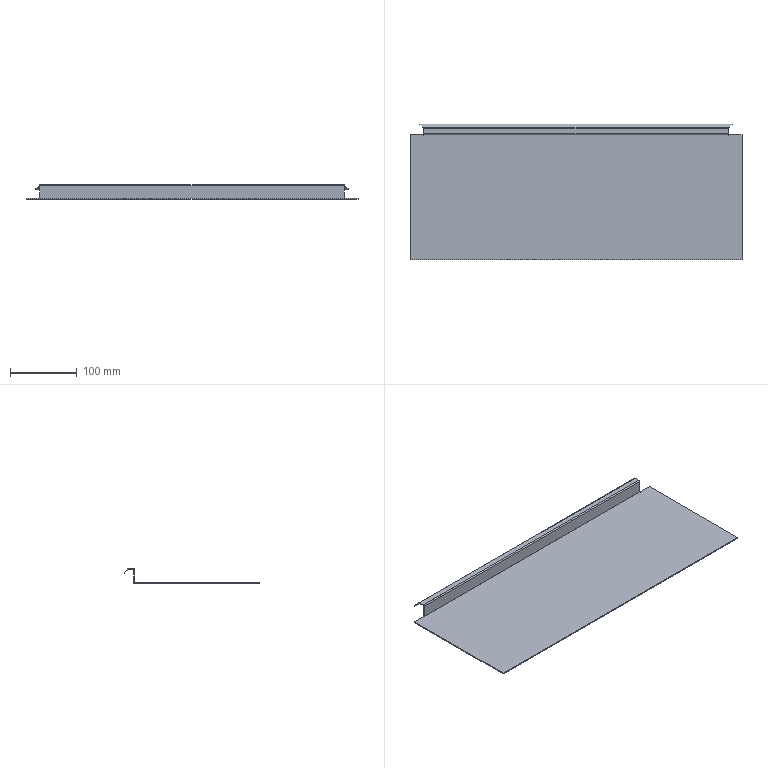Part | SolidWorks | features EdgeFlange 3, SMBaseFlange 2, FlatPattern 1, SheetMetal 1 | 1 solid | 40 faces | box 496.5 x 203.157 x 22 mm | volume 165083 mm3 | plane 34 | cylinder 6 | commonest cylinder face diameters 0.2 x3 3.2 x3
STEP:
#1=CARTESIAN_POINT('',(227.95,103.087,19.));
#2=VERTEX_POINT('',#1);
#3=CARTESIAN_POINT('',(227.95,103.087,20.5));
#4=VERTEX_POINT('',#3);
#5=CARTESIAN_POINT('',(227.95,103.087,19.));
#6=DIRECTION('',(0.,0.,1.));
#7=VECTOR('',#6,1000.);
#8=LINE('',#5,#7);
#9=EDGE_CURVE('',#2,#4,#8,.T.);
#10=ORIENTED_EDGE('',*,*,#9,.T.);
#11=CARTESIAN_POINT('',(227.95,95.35,20.5));
#12=VERTEX_POINT('',#11);
#13=CARTESIAN_POINT('',(227.95,95.25,20.5));
#14=DIRECTION('',(0.,1.,0.));
#15=VECTOR('',#14,1000.);
#16=LINE('',#13,#15);
#17=EDGE_CURVE('',#12,#4,#16,.T.);
#18=ORIENTED_EDGE('',*,*,#17,.F.);
#19=CARTESIAN_POINT('',(227.95,95.35,19.));
#20=VERTEX_POINT('',#19);
#21=CARTESIAN_POINT('',(227.95,95.35,19.));
#22=DIRECTION('',(0.,0.,1.));
#23=VECTOR('',#22,1000.);
#24=LINE('',#21,#23);
#25=EDGE_CURVE('',#20,#12,#24,.T.);
#26=ORIENTED_EDGE('',*,*,#25,.F.);
#27=CARTESIAN_POINT('',(227.95,103.75,19.));
#28=DIRECTION('',(0.,1.,0.));
#29=VECTOR('',#28,1000.);
#30=LINE('',#27,#29);
#31=EDGE_CURVE('',#20,#2,#30,.T.);
#32=ORIENTED_EDGE('',*,*,#31,.T.);
#33=EDGE_LOOP('',(#10,#18,#26,#32));
#34=FACE_OUTER_BOUND('',#33,.T.);
#35=CARTESIAN_POINT('',(227.95,103.75,20.5));
#36=DIRECTION('',(-1.,0.,0.));
#37=DIRECTION('',(0.,0.,1.));
#38=AXIS2_PLACEMENT_3D('',#35,#36,#37);
#39=PLANE('',#38);
#40=ADVANCED_FACE('',(#34),#39,.F.);
#41=CARTESIAN_POINT('',(-227.95,103.087,19.));
#42=VERTEX_POINT('',#41);
#43=CARTESIAN_POINT('',(-227.95,103.087,20.5));
#44=VERTEX_POINT('',#43);
#45=CARTESIAN_POINT('',(-227.95,103.087,19.));
#46=DIRECTION('',(0.,0.,1.));
#47=VECTOR('',#46,1000.);
#48=LINE('',#45,#47);
#49=EDGE_CURVE('',#42,#44,#48,.T.);
#50=ORIENTED_EDGE('',*,*,#49,.F.);
#51=CARTESIAN_POINT('',(-227.95,95.35,19.));
#52=VERTEX_POINT('',#51);
#53=CARTESIAN_POINT('',(-227.95,95.25,19.));
#54=DIRECTION('',(0.,-1.,0.));
#55=VECTOR('',#54,1000.);
#56=LINE('',#53,#55);
#57=EDGE_CURVE('',#42,#52,#56,.T.);
#58=ORIENTED_EDGE('',*,*,#57,.T.);
#59=CARTESIAN_POINT('',(-227.95,95.35,20.5));
#60=VERTEX_POINT('',#59);
#61=CARTESIAN_POINT('',(-227.95,95.35,20.5));
#62=DIRECTION('',(0.,0.,1.));
#63=VECTOR('',#62,1000.);
#64=LINE('',#61,#63);
#65=EDGE_CURVE('',#52,#60,#64,.T.);
#66=ORIENTED_EDGE('',*,*,#65,.T.);
#67=CARTESIAN_POINT('',(-227.95,95.25,20.5));
#68=DIRECTION('',(0.,-1.,0.));
#69=VECTOR('',#68,1000.);
#70=LINE('',#67,#69);
#71=EDGE_CURVE('',#44,#60,#70,.T.);
#72=ORIENTED_EDGE('',*,*,#71,.F.);
#73=EDGE_LOOP('',(#50,#58,#66,#72));
#74=FACE_OUTER_BOUND('',#73,.T.);
#75=CARTESIAN_POINT('',(-227.95,95.25,20.5));
#76=DIRECTION('',(1.,0.,0.));
#77=DIRECTION('',(0.,0.,-1.));
#78=AXIS2_PLACEMENT_3D('',#75,#76,#77);
#79=PLANE('',#78);
#80=ADVANCED_FACE('',(#74),#79,.F.);
#81=CARTESIAN_POINT('',(227.95,103.087,20.5));
#82=DIRECTION('',(-1.,0.,0.));
#83=VECTOR('',#82,1000.);
#84=LINE('',#81,#83);
#85=EDGE_CURVE('',#4,#44,#84,.T.);
#86=ORIENTED_EDGE('',*,*,#85,.T.);
#87=ORIENTED_EDGE('',*,*,#71,.T.);
#88=CARTESIAN_POINT('',(-227.95,95.35,20.5));
#89=DIRECTION('',(-1.,0.,0.));
#90=VECTOR('',#89,1000.);
#91=LINE('',#88,#90);
#92=EDGE_CURVE('',#12,#60,#91,.T.);
#93=ORIENTED_EDGE('',*,*,#92,.F.);
#94=ORIENTED_EDGE('',*,*,#17,.T.);
#95=EDGE_LOOP('',(#86,#87,#93,#94));
#96=FACE_OUTER_BOUND('',#95,.T.);
#97=CARTESIAN_POINT('',(-227.95,95.25,20.5));
#98=DIRECTION('',(0.,0.,-1.));
#99=DIRECTION('',(-1.,0.,0.));
#100=AXIS2_PLACEMENT_3D('',#97,#98,#99);
#101=PLANE('',#100);
#102=ADVANCED_FACE('',(#96),#101,.F.);
#103=ORIENTED_EDGE('',*,*,#57,.F.);
#104=CARTESIAN_POINT('',(227.95,103.087,19.));
#105=DIRECTION('',(-1.,0.,0.));
#106=VECTOR('',#105,1000.);
#107=LINE('',#104,#106);
#108=EDGE_CURVE('',#2,#42,#107,.T.);
#109=ORIENTED_EDGE('',*,*,#108,.F.);
#110=ORIENTED_EDGE('',*,*,#31,.F.);
#111=CARTESIAN_POINT('',(-227.95,95.35,19.));
#112=DIRECTION('',(1.,0.,0.));
#113=VECTOR('',#112,1000.);
#114=LINE('',#111,#113);
#115=EDGE_CURVE('',#52,#20,#114,.T.);
#116=ORIENTED_EDGE('',*,*,#115,.F.);
#117=EDGE_LOOP('',(#103,#109,#110,#116));
#118=FACE_OUTER_BOUND('',#117,.T.);
#119=CARTESIAN_POINT('',(-227.95,95.25,19.));
#120=DIRECTION('',(0.,0.,-1.));
#121=DIRECTION('',(-1.,0.,0.));
#122=AXIS2_PLACEMENT_3D('',#119,#120,#121);
#123=PLANE('',#122);
#124=ADVANCED_FACE('',(#118),#123,.T.);
#125=CARTESIAN_POINT('',(227.95,95.25,0.1));
#126=VERTEX_POINT('',#125);
#127=CARTESIAN_POINT('',(227.95,95.25,18.9));
#128=VERTEX_POINT('',#127);
#129=CARTESIAN_POINT('',(227.95,95.25,20.5));
#130=DIRECTION('',(0.,0.,1.));
#131=VECTOR('',#130,1000.);
#132=LINE('',#129,#131);
#133=EDGE_CURVE('',#126,#128,#132,.T.);
#134=ORIENTED_EDGE('',*,*,#133,.T.);
#135=CARTESIAN_POINT('',(227.95,93.75,18.9));
#136=VERTEX_POINT('',#135);
#137=CARTESIAN_POINT('',(227.95,95.25,18.9));
#138=DIRECTION('',(0.,-1.,0.));
#139=VECTOR('',#138,1000.);
#140=LINE('',#137,#139);
#141=EDGE_CURVE('',#128,#136,#140,.T.);
#142=ORIENTED_EDGE('',*,*,#141,.T.);
#143=CARTESIAN_POINT('',(227.95,93.75,0.1));
#144=VERTEX_POINT('',#143);
#145=CARTESIAN_POINT('',(227.95,93.75,20.5));
#146=DIRECTION('',(0.,0.,1.));
#147=VECTOR('',#146,1000.);
#148=LINE('',#145,#147);
#149=EDGE_CURVE('',#144,#136,#148,.T.);
#150=ORIENTED_EDGE('',*,*,#149,.F.);
#151=CARTESIAN_POINT('',(227.95,93.75,0.1));
#152=DIRECTION('',(0.,1.,0.));
#153=VECTOR('',#152,1000.);
#154=LINE('',#151,#153);
#155=EDGE_CURVE('',#144,#126,#154,.T.);
#156=ORIENTED_EDGE('',*,*,#155,.T.);
#157=EDGE_LOOP('',(#134,#142,#150,#156));
#158=FACE_OUTER_BOUND('',#157,.T.);
#159=CARTESIAN_POINT('',(227.95,95.25,20.5));
#160=DIRECTION('',(1.,0.,0.));
#161=DIRECTION('',(0.,0.,-1.));
#162=AXIS2_PLACEMENT_3D('',#159,#160,#161);
#163=PLANE('',#162);
#164=ADVANCED_FACE('',(#158),#163,.T.);
#165=CARTESIAN_POINT('',(-227.95,95.25,18.9));
#166=VERTEX_POINT('',#165);
#167=CARTESIAN_POINT('',(-227.95,95.25,0.1));
#168=VERTEX_POINT('',#167);
#169=CARTESIAN_POINT('',(-227.95,95.25,0.));
#170=DIRECTION('',(0.,0.,-1.));
#171=VECTOR('',#170,1000.);
#172=LINE('',#169,#171);
#173=EDGE_CURVE('',#166,#168,#172,.T.);
#174=ORIENTED_EDGE('',*,*,#173,.F.);
#175=CARTESIAN_POINT('',(227.95,95.25,18.9));
#176=DIRECTION('',(-1.,0.,0.));
#177=VECTOR('',#176,1000.);
#178=LINE('',#175,#177);
#179=EDGE_CURVE('',#128,#166,#178,.T.);
#180=ORIENTED_EDGE('',*,*,#179,.F.);
#181=ORIENTED_EDGE('',*,*,#133,.F.);
#182=CARTESIAN_POINT('',(-227.95,95.25,0.1));
#183=DIRECTION('',(-1.,0.,0.));
#184=VECTOR('',#183,1000.);
#185=LINE('',#182,#184);
#186=EDGE_CURVE('',#126,#168,#185,.T.);
#187=ORIENTED_EDGE('',*,*,#186,.T.);
#188=EDGE_LOOP('',(#174,#180,#181,#187));
#189=FACE_OUTER_BOUND('',#188,.T.);
#190=CARTESIAN_POINT('',(-227.95,95.25,0.));
#191=DIRECTION('',(0.,1.,0.));
#192=DIRECTION('',(0.,0.,1.));
#193=AXIS2_PLACEMENT_3D('',#190,#191,#192);
#194=PLANE('',#193);
#195=ADVANCED_FACE('',(#189),#194,.T.);
#196=CARTESIAN_POINT('',(-227.95,93.75,18.9));
#197=VERTEX_POINT('',#196);
#198=CARTESIAN_POINT('',(227.95,93.75,18.9));
#199=DIRECTION('',(-1.,0.,0.));
#200=VECTOR('',#199,1000.);
#201=LINE('',#198,#200);
#202=EDGE_CURVE('',#136,#197,#201,.T.);
#203=ORIENTED_EDGE('',*,*,#202,.T.);
#204=CARTESIAN_POINT('',(-227.95,93.75,0.1));
#205=VERTEX_POINT('',#204);
#206=CARTESIAN_POINT('',(-227.95,93.75,0.));
#207=DIRECTION('',(0.,0.,-1.));
#208=VECTOR('',#207,1000.);
#209=LINE('',#206,#208);
#210=EDGE_CURVE('',#197,#205,#209,.T.);
#211=ORIENTED_EDGE('',*,*,#210,.T.);
#212=CARTESIAN_POINT('',(227.95,93.75,0.1));
#213=DIRECTION('',(-1.,0.,0.));
#214=VECTOR('',#213,1000.);
#215=LINE('',#212,#214);
#216=EDGE_CURVE('',#144,#205,#215,.T.);
#217=ORIENTED_EDGE('',*,*,#216,.F.);
#218=ORIENTED_EDGE('',*,*,#149,.T.);
#219=EDGE_LOOP('',(#203,#211,#217,#218));
#220=FACE_OUTER_BOUND('',#219,.T.);
#221=CARTESIAN_POINT('',(-227.95,93.75,0.));
#222=DIRECTION('',(0.,1.,0.));
#223=DIRECTION('',(0.,0.,1.));
#224=AXIS2_PLACEMENT_3D('',#221,#222,#223);
#225=PLANE('',#224);
#226=ADVANCED_FACE('',(#220),#225,.F.);
#227=CARTESIAN_POINT('',(-228.7,93.75,0.));
#228=VERTEX_POINT('',#227);
#229=CARTESIAN_POINT('',(-248.25,93.75,0.));
#230=VERTEX_POINT('',#229);
#231=CARTESIAN_POINT('',(-248.25,93.75,0.));
#232=DIRECTION('',(-1.,0.,0.));
#233=VECTOR('',#232,1000.);
#234=LINE('',#231,#233);
#235=EDGE_CURVE('',#228,#230,#234,.T.);
#236=ORIENTED_EDGE('',*,*,#235,.F.);
#237=CARTESIAN_POINT('',(-228.7,93.75,-1.5));
#238=VERTEX_POINT('',#237);
#239=CARTESIAN_POINT('',(-228.7,93.75,0.));
#240=DIRECTION('',(0.,0.,-1.));
#241=VECTOR('',#240,1000.);
#242=LINE('',#239,#241);
#243=EDGE_CURVE('',#228,#238,#242,.T.);
#244=ORIENTED_EDGE('',*,*,#243,.T.);
#245=CARTESIAN_POINT('',(-248.25,93.75,-1.5));
#246=VERTEX_POINT('',#245);
#247=CARTESIAN_POINT('',(-248.25,93.75,-1.5));
#248=DIRECTION('',(-1.,0.,0.));
#249=VECTOR('',#248,1000.);
#250=LINE('',#247,#249);
#251=EDGE_CURVE('',#238,#246,#250,.T.);
#252=ORIENTED_EDGE('',*,*,#251,.T.);
#253=CARTESIAN_POINT('',(-248.25,93.75,-1.5));
#254=DIRECTION('',(0.,0.,1.));
#255=VECTOR('',#254,1000.);
#256=LINE('',#253,#255);
#257=EDGE_CURVE('',#246,#230,#256,.T.);
#258=ORIENTED_EDGE('',*,*,#257,.T.);
#259=EDGE_LOOP('',(#236,#244,#252,#258));
#260=FACE_OUTER_BOUND('',#259,.T.);
#261=CARTESIAN_POINT('',(-248.25,93.75,-1.5));
#262=DIRECTION('',(0.,1.,0.));
#263=DIRECTION('',(0.,0.,1.));
#264=AXIS2_PLACEMENT_3D('',#261,#262,#263);
#265=PLANE('',#264);
#266=ADVANCED_FACE('',(#260),#265,.T.);
#267=CARTESIAN_POINT('',(248.25,93.75,-1.5));
#268=VERTEX_POINT('',#267);
#269=CARTESIAN_POINT('',(228.7,93.75,-1.5));
#270=VERTEX_POINT('',#269);
#271=CARTESIAN_POINT('',(-248.25,93.75,-1.5));
#272=DIRECTION('',(-1.,0.,0.));
#273=VECTOR('',#272,1000.);
#274=LINE('',#271,#273);
#275=EDGE_CURVE('',#268,#270,#274,.T.);
#276=ORIENTED_EDGE('',*,*,#275,.T.);
#277=CARTESIAN_POINT('',(228.7,93.75,0.));
#278=VERTEX_POINT('',#277);
#279=CARTESIAN_POINT('',(228.7,93.75,0.));
#280=DIRECTION('',(0.,0.,-1.));
#281=VECTOR('',#280,1000.);
#282=LINE('',#279,#281);
#283=EDGE_CURVE('',#278,#270,#282,.T.);
#284=ORIENTED_EDGE('',*,*,#283,.F.);
#285=CARTESIAN_POINT('',(248.25,93.75,0.));
#286=VERTEX_POINT('',#285);
#287=CARTESIAN_POINT('',(-248.25,93.75,0.));
#288=DIRECTION('',(-1.,0.,0.));
#289=VECTOR('',#288,1000.);
#290=LINE('',#287,#289);
#291=EDGE_CURVE('',#286,#278,#290,.T.);
#292=ORIENTED_EDGE('',*,*,#291,.F.);
#293=CARTESIAN_POINT('',(248.25,93.75,-1.5));
#294=DIRECTION('',(0.,0.,1.));
#295=VECTOR('',#294,1000.);
#296=LINE('',#293,#295);
#297=EDGE_CURVE('',#268,#286,#296,.T.);
#298=ORIENTED_EDGE('',*,*,#297,.F.);
#299=EDGE_LOOP('',(#276,#284,#292,#298));
#300=FACE_OUTER_BOUND('',#299,.T.);
#301=CARTESIAN_POINT('',(-248.25,93.75,-1.5));
#302=DIRECTION('',(0.,1.,0.));
#303=DIRECTION('',(0.,0.,1.));
#304=AXIS2_PLACEMENT_3D('',#301,#302,#303);
#305=PLANE('',#304);
#306=ADVANCED_FACE('',(#300),#305,.T.);
#307=CARTESIAN_POINT('',(-228.7,92.9,-1.5));
#308=VERTEX_POINT('',#307);
#309=CARTESIAN_POINT('',(-228.7,-93.75,-1.5));
#310=DIRECTION('',(0.,1.,0.));
#311=VECTOR('',#310,1000.);
#312=LINE('',#309,#311);
#313=EDGE_CURVE('',#308,#238,#312,.T.);
#314=ORIENTED_EDGE('',*,*,#313,.F.);
#315=CARTESIAN_POINT('',(-227.95,92.9,-1.5));
#316=VERTEX_POINT('',#315);
#317=CARTESIAN_POINT('',(248.25,92.9,-1.5));
#318=DIRECTION('',(-1.,0.,0.));
#319=VECTOR('',#318,1000.);
#320=LINE('',#317,#319);
#321=EDGE_CURVE('',#316,#308,#320,.T.);
#322=ORIENTED_EDGE('',*,*,#321,.F.);
#323=CARTESIAN_POINT('',(-227.95,93.65,-1.5));
#324=VERTEX_POINT('',#323);
#325=CARTESIAN_POINT('',(-227.95,-93.75,-1.5));
#326=DIRECTION('',(0.,-1.,0.));
#327=VECTOR('',#326,1000.);
#328=LINE('',#325,#327);
#329=EDGE_CURVE('',#324,#316,#328,.T.);
#330=ORIENTED_EDGE('',*,*,#329,.F.);
#331=CARTESIAN_POINT('',(227.95,93.65,-1.5));
#332=VERTEX_POINT('',#331);
#333=CARTESIAN_POINT('',(-227.95,93.65,-1.5));
#334=DIRECTION('',(1.,0.,0.));
#335=VECTOR('',#334,1000.);
#336=LINE('',#333,#335);
#337=EDGE_CURVE('',#324,#332,#336,.T.);
#338=ORIENTED_EDGE('',*,*,#337,.T.);
#339=CARTESIAN_POINT('',(227.95,92.9,-1.5));
#340=VERTEX_POINT('',#339);
#341=CARTESIAN_POINT('',(227.95,-93.75,-1.5));
#342=DIRECTION('',(0.,1.,0.));
#343=VECTOR('',#342,1000.);
#344=LINE('',#341,#343);
#345=EDGE_CURVE('',#340,#332,#344,.T.);
#346=ORIENTED_EDGE('',*,*,#345,.F.);
#347=CARTESIAN_POINT('',(228.7,92.9,-1.5));
#348=VERTEX_POINT('',#347);
#349=CARTESIAN_POINT('',(248.25,92.9,-1.5));
#350=DIRECTION('',(-1.,0.,0.));
#351=VECTOR('',#350,1000.);
#352=LINE('',#349,#351);
#353=EDGE_CURVE('',#348,#340,#352,.T.);
#354=ORIENTED_EDGE('',*,*,#353,.F.);
#355=CARTESIAN_POINT('',(228.7,-93.75,-1.5));
#356=DIRECTION('',(0.,-1.,0.));
#357=VECTOR('',#356,1000.);
#358=LINE('',#355,#357);
#359=EDGE_CURVE('',#270,#348,#358,.T.);
#360=ORIENTED_EDGE('',*,*,#359,.F.);
#361=ORIENTED_EDGE('',*,*,#275,.F.);
#362=CARTESIAN_POINT('',(248.25,-93.75,-1.5));
#363=VERTEX_POINT('',#362);
#364=CARTESIAN_POINT('',(248.25,93.75,-1.5));
#365=DIRECTION('',(0.,1.,0.));
#366=VECTOR('',#365,1000.);
#367=LINE('',#364,#366);
#368=EDGE_CURVE('',#363,#268,#367,.T.);
#369=ORIENTED_EDGE('',*,*,#368,.F.);
#370=CARTESIAN_POINT('',(-248.25,-93.75,-1.5));
#371=VERTEX_POINT('',#370);
#372=CARTESIAN_POINT('',(-248.25,-93.75,-1.5));
#373=DIRECTION('',(1.,0.,0.));
#374=VECTOR('',#373,1000.);
#375=LINE('',#372,#374);
#376=EDGE_CURVE('',#371,#363,#375,.T.);
#377=ORIENTED_EDGE('',*,*,#376,.F.);
#378=CARTESIAN_POINT('',(-248.25,93.75,-1.5));
#379=DIRECTION('',(0.,-1.,0.));
#380=VECTOR('',#379,1000.);
#381=LINE('',#378,#380);
#382=EDGE_CURVE('',#246,#371,#381,.T.);
#383=ORIENTED_EDGE('',*,*,#382,.F.);
#384=ORIENTED_EDGE('',*,*,#251,.F.);
#385=EDGE_LOOP('',(#314,#322,#330,#338,#346,#354,#360,#361,#369,#377,#383,#384));
#386=FACE_OUTER_BOUND('',#385,.T.);
#387=CARTESIAN_POINT('',(248.25,-93.75,-1.5));
#388=DIRECTION('',(0.,0.,1.));
#389=DIRECTION('',(1.,0.,0.));
#390=AXIS2_PLACEMENT_3D('',#387,#388,#389);
#391=PLANE('',#390);
#392=ADVANCED_FACE('',(#386),#391,.F.);
#393=CARTESIAN_POINT('',(-228.7,92.9,0.));
#394=VERTEX_POINT('',#393);
#395=CARTESIAN_POINT('',(-227.95,92.9,0.));
#396=VERTEX_POINT('',#395);
#397=CARTESIAN_POINT('',(-228.7,92.9,0.));
#398=DIRECTION('',(1.,0.,0.));
#399=VECTOR('',#398,1000.);
#400=LINE('',#397,#399);
#401=EDGE_CURVE('',#394,#396,#400,.T.);
#402=ORIENTED_EDGE('',*,*,#401,.F.);
#403=CARTESIAN_POINT('',(-228.7,93.75,0.));
#404=DIRECTION('',(0.,-1.,0.));
#405=VECTOR('',#404,1000.);
#406=LINE('',#403,#405);
#407=EDGE_CURVE('',#228,#394,#406,.T.);
#408=ORIENTED_EDGE('',*,*,#407,.F.);
#409=ORIENTED_EDGE('',*,*,#235,.T.);
#410=CARTESIAN_POINT('',(-248.25,-93.75,0.));
#411=VERTEX_POINT('',#410);
#412=CARTESIAN_POINT('',(-248.25,93.75,0.));
#413=DIRECTION('',(0.,-1.,0.));
#414=VECTOR('',#413,1000.);
#415=LINE('',#412,#414);
#416=EDGE_CURVE('',#230,#411,#415,.T.);
#417=ORIENTED_EDGE('',*,*,#416,.T.);
#418=CARTESIAN_POINT('',(248.25,-93.75,0.));
#419=VERTEX_POINT('',#418);
#420=CARTESIAN_POINT('',(-248.25,-93.75,0.));
#421=DIRECTION('',(1.,0.,0.));
#422=VECTOR('',#421,1000.);
#423=LINE('',#420,#422);
#424=EDGE_CURVE('',#411,#419,#423,.T.);
#425=ORIENTED_EDGE('',*,*,#424,.T.);
#426=CARTESIAN_POINT('',(248.25,93.75,0.));
#427=DIRECTION('',(0.,1.,0.));
#428=VECTOR('',#427,1000.);
#429=LINE('',#426,#428);
#430=EDGE_CURVE('',#419,#286,#429,.T.);
#431=ORIENTED_EDGE('',*,*,#430,.T.);
#432=ORIENTED_EDGE('',*,*,#291,.T.);
#433=CARTESIAN_POINT('',(228.7,92.9,0.));
#434=VERTEX_POINT('',#433);
#435=CARTESIAN_POINT('',(228.7,92.9,0.));
#436=DIRECTION('',(0.,1.,0.));
#437=VECTOR('',#436,1000.);
#438=LINE('',#435,#437);
#439=EDGE_CURVE('',#434,#278,#438,.T.);
#440=ORIENTED_EDGE('',*,*,#439,.F.);
#441=CARTESIAN_POINT('',(227.95,92.9,0.));
#442=VERTEX_POINT('',#441);
#443=CARTESIAN_POINT('',(227.95,92.9,0.));
#444=DIRECTION('',(1.,0.,0.));
#445=VECTOR('',#444,1000.);
#446=LINE('',#443,#445);
#447=EDGE_CURVE('',#442,#434,#446,.T.);
#448=ORIENTED_EDGE('',*,*,#447,.F.);
#449=CARTESIAN_POINT('',(227.95,93.65,0.));
#450=VERTEX_POINT('',#449);
#451=CARTESIAN_POINT('',(227.95,93.65,0.));
#452=DIRECTION('',(0.,-1.,0.));
#453=VECTOR('',#452,1000.);
#454=LINE('',#451,#453);
#455=EDGE_CURVE('',#450,#442,#454,.T.);
#456=ORIENTED_EDGE('',*,*,#455,.F.);
#457=CARTESIAN_POINT('',(-227.95,93.65,0.));
#458=VERTEX_POINT('',#457);
#459=CARTESIAN_POINT('',(-227.95,93.65,0.));
#460=DIRECTION('',(1.,0.,0.));
#461=VECTOR('',#460,1000.);
#462=LINE('',#459,#461);
#463=EDGE_CURVE('',#458,#450,#462,.T.);
#464=ORIENTED_EDGE('',*,*,#463,.F.);
#465=CARTESIAN_POINT('',(-227.95,92.9,0.));
#466=DIRECTION('',(0.,1.,0.));
#467=VECTOR('',#466,1000.);
#468=LINE('',#465,#467);
#469=EDGE_CURVE('',#396,#458,#468,.T.);
#470=ORIENTED_EDGE('',*,*,#469,.F.);
#471=EDGE_LOOP('',(#402,#408,#409,#417,#425,#431,#432,#440,#448,#456,#464,#470));
#472=FACE_OUTER_BOUND('',#471,.T.);
#473=CARTESIAN_POINT('',(248.25,-93.75,0.));
#474=DIRECTION('',(0.,0.,1.));
#475=DIRECTION('',(1.,0.,0.));
#476=AXIS2_PLACEMENT_3D('',#473,#474,#475);
#477=PLANE('',#476);
#478=ADVANCED_FACE('',(#472),#477,.T.);
#479=ORIENTED_EDGE('',*,*,#430,.F.);
#480=CARTESIAN_POINT('',(248.25,-93.75,-1.5));
#481=DIRECTION('',(0.,0.,1.));
#482=VECTOR('',#481,1000.);
#483=LINE('',#480,#482);
#484=EDGE_CURVE('',#363,#419,#483,.T.);
#485=ORIENTED_EDGE('',*,*,#484,.F.);
#486=ORIENTED_EDGE('',*,*,#368,.T.);
#487=ORIENTED_EDGE('',*,*,#297,.T.);
#488=EDGE_LOOP('',(#479,#485,#486,#487));
#489=FACE_OUTER_BOUND('',#488,.T.);
#490=CARTESIAN_POINT('',(248.25,93.75,-1.5));
#491=DIRECTION('',(1.,0.,0.));
#492=DIRECTION('',(0.,0.,-1.));
#493=AXIS2_PLACEMENT_3D('',#490,#491,#492);
#494=PLANE('',#493);
#495=ADVANCED_FACE('',(#489),#494,.T.);
#496=ORIENTED_EDGE('',*,*,#424,.F.);
#497=CARTESIAN_POINT('',(-248.25,-93.75,-1.5));
#498=DIRECTION('',(0.,0.,1.));
#499=VECTOR('',#498,1000.);
#500=LINE('',#497,#499);
#501=EDGE_CURVE('',#371,#411,#500,.T.);
#502=ORIENTED_EDGE('',*,*,#501,.F.);
#503=ORIENTED_EDGE('',*,*,#376,.T.);
#504=ORIENTED_EDGE('',*,*,#484,.T.);
#505=EDGE_LOOP('',(#496,#502,#503,#504));
#506=FACE_OUTER_BOUND('',#505,.T.);
#507=CARTESIAN_POINT('',(-248.25,-93.75,-1.5));
#508=DIRECTION('',(0.,-1.,0.));
#509=DIRECTION('',(0.,0.,-1.));
#510=AXIS2_PLACEMENT_3D('',#507,#508,#509);
#511=PLANE('',#510);
#512=ADVANCED_FACE('',(#506),#511,.T.);
#513=ORIENTED_EDGE('',*,*,#416,.F.);
#514=ORIENTED_EDGE('',*,*,#257,.F.);
#515=ORIENTED_EDGE('',*,*,#382,.T.);
#516=ORIENTED_EDGE('',*,*,#501,.T.);
#517=EDGE_LOOP('',(#513,#514,#515,#516));
#518=FACE_OUTER_BOUND('',#517,.T.);
#519=CARTESIAN_POINT('',(-248.25,93.75,-1.5));
#520=DIRECTION('',(-1.,0.,0.));
#521=DIRECTION('',(0.,-1.,0.));
#522=AXIS2_PLACEMENT_3D('',#519,#520,#521);
#523=PLANE('',#522);
#524=ADVANCED_FACE('',(#518),#523,.T.);
#525=CARTESIAN_POINT('',(-228.7,92.9,0.));
#526=DIRECTION('',(0.,0.,-1.));
#527=VECTOR('',#526,1000.);
#528=LINE('',#525,#527);
#529=EDGE_CURVE('',#394,#308,#528,.T.);
#530=ORIENTED_EDGE('',*,*,#529,.T.);
#531=ORIENTED_EDGE('',*,*,#313,.T.);
#532=ORIENTED_EDGE('',*,*,#243,.F.);
#533=ORIENTED_EDGE('',*,*,#407,.T.);
#534=EDGE_LOOP('',(#530,#531,#532,#533));
#535=FACE_OUTER_BOUND('',#534,.T.);
#536=CARTESIAN_POINT('',(-228.7,93.75,0.));
#537=DIRECTION('',(1.,0.,0.));
#538=DIRECTION('',(0.,0.,-1.));
#539=AXIS2_PLACEMENT_3D('',#536,#537,#538);
#540=PLANE('',#539);
#541=ADVANCED_FACE('',(#535),#540,.T.);
#542=CARTESIAN_POINT('',(-227.95,92.9,0.));
#543=DIRECTION('',(0.,0.,-1.));
#544=VECTOR('',#543,1000.);
#545=LINE('',#542,#544);
#546=EDGE_CURVE('',#396,#316,#545,.T.);
#547=ORIENTED_EDGE('',*,*,#546,.T.);
#548=ORIENTED_EDGE('',*,*,#321,.T.);
#549=ORIENTED_EDGE('',*,*,#529,.F.);
#550=ORIENTED_EDGE('',*,*,#401,.T.);
#551=EDGE_LOOP('',(#547,#548,#549,#550));
#552=FACE_OUTER_BOUND('',#551,.T.);
#553=CARTESIAN_POINT('',(-228.7,92.9,0.));
#554=DIRECTION('',(0.,1.,0.));
#555=DIRECTION('',(0.,0.,1.));
#556=AXIS2_PLACEMENT_3D('',#553,#554,#555);
#557=PLANE('',#556);
#558=ADVANCED_FACE('',(#552),#557,.T.);
#559=CARTESIAN_POINT('',(-227.95,93.65,0.));
#560=DIRECTION('',(0.,0.,-1.));
#561=VECTOR('',#560,1000.);
#562=LINE('',#559,#561);
#563=EDGE_CURVE('',#458,#324,#562,.T.);
#564=ORIENTED_EDGE('',*,*,#563,.T.);
#565=ORIENTED_EDGE('',*,*,#329,.T.);
#566=ORIENTED_EDGE('',*,*,#546,.F.);
#567=ORIENTED_EDGE('',*,*,#469,.T.);
#568=EDGE_LOOP('',(#564,#565,#566,#567));
#569=FACE_OUTER_BOUND('',#568,.T.);
#570=CARTESIAN_POINT('',(-227.95,92.9,0.));
#571=DIRECTION('',(-1.,0.,0.));
#572=DIRECTION('',(0.,0.,1.));
#573=AXIS2_PLACEMENT_3D('',#570,#571,#572);
#574=PLANE('',#573);
#575=ADVANCED_FACE('',(#569),#574,.T.);
#576=CARTESIAN_POINT('',(227.95,92.9,0.));
#577=DIRECTION('',(0.,0.,-1.));
#578=VECTOR('',#577,1000.);
#579=LINE('',#576,#578);
#580=EDGE_CURVE('',#442,#340,#579,.T.);
#581=ORIENTED_EDGE('',*,*,#580,.T.);
#582=ORIENTED_EDGE('',*,*,#345,.T.);
#583=CARTESIAN_POINT('',(227.95,93.65,0.));
#584=DIRECTION('',(0.,0.,-1.));
#585=VECTOR('',#584,1000.);
#586=LINE('',#583,#585);
#587=EDGE_CURVE('',#450,#332,#586,.T.);
#588=ORIENTED_EDGE('',*,*,#587,.F.);
#589=ORIENTED_EDGE('',*,*,#455,.T.);
#590=EDGE_LOOP('',(#581,#582,#588,#589));
#591=FACE_OUTER_BOUND('',#590,.T.);
#592=CARTESIAN_POINT('',(227.95,93.65,0.));
#593=DIRECTION('',(1.,0.,0.));
#594=DIRECTION('',(0.,0.,-1.));
#595=AXIS2_PLACEMENT_3D('',#592,#593,#594);
#596=PLANE('',#595);
#597=ADVANCED_FACE('',(#591),#596,.T.);
#598=CARTESIAN_POINT('',(228.7,92.9,0.));
#599=DIRECTION('',(0.,0.,-1.));
#600=VECTOR('',#599,1000.);
#601=LINE('',#598,#600);
#602=EDGE_CURVE('',#434,#348,#601,.T.);
#603=ORIENTED_EDGE('',*,*,#602,.T.);
#604=ORIENTED_EDGE('',*,*,#353,.T.);
#605=ORIENTED_EDGE('',*,*,#580,.F.);
#606=ORIENTED_EDGE('',*,*,#447,.T.);
#607=EDGE_LOOP('',(#603,#604,#605,#606));
#608=FACE_OUTER_BOUND('',#607,.T.);
#609=CARTESIAN_POINT('',(227.95,92.9,0.));
#610=DIRECTION('',(0.,1.,0.));
#611=DIRECTION('',(0.,0.,1.));
#612=AXIS2_PLACEMENT_3D('',#609,#610,#611);
#613=PLANE('',#612);
#614=ADVANCED_FACE('',(#608),#613,.T.);
#615=ORIENTED_EDGE('',*,*,#283,.T.);
#616=ORIENTED_EDGE('',*,*,#359,.T.);
#617=ORIENTED_EDGE('',*,*,#602,.F.);
#618=ORIENTED_EDGE('',*,*,#439,.T.);
#619=EDGE_LOOP('',(#615,#616,#617,#618));
#620=FACE_OUTER_BOUND('',#619,.T.);
#621=CARTESIAN_POINT('',(228.7,92.9,0.));
#622=DIRECTION('',(-1.,0.,0.));
#623=DIRECTION('',(0.,0.,1.));
#624=AXIS2_PLACEMENT_3D('',#621,#622,#623);
#625=PLANE('',#624);
#626=ADVANCED_FACE('',(#620),#625,.T.);
#627=ORIENTED_EDGE('',*,*,#155,.F.);
#628=CARTESIAN_POINT('',(227.95,93.65,0.1));
#629=DIRECTION('',(1.,0.,0.));
#630=DIRECTION('',(0.,0.,1.));
#631=AXIS2_PLACEMENT_3D('',#628,#629,#630);
#632=CIRCLE('',#631,0.1);
#633=EDGE_CURVE('',#450,#144,#632,.T.);
#634=ORIENTED_EDGE('',*,*,#633,.F.);
#635=ORIENTED_EDGE('',*,*,#587,.T.);
#636=CARTESIAN_POINT('',(227.95,93.65,0.1));
#637=DIRECTION('',(1.,0.,0.));
#638=DIRECTION('',(0.,0.,1.));
#639=AXIS2_PLACEMENT_3D('',#636,#637,#638);
#640=CIRCLE('',#639,1.6);
#641=EDGE_CURVE('',#332,#126,#640,.T.);
#642=ORIENTED_EDGE('',*,*,#641,.T.);
#643=EDGE_LOOP('',(#627,#634,#635,#642));
#644=FACE_OUTER_BOUND('',#643,.T.);
#645=CARTESIAN_POINT('',(227.95,93.65,0.1));
#646=DIRECTION('',(1.,0.,0.));
#647=DIRECTION('',(0.,0.,-1.));
#648=AXIS2_PLACEMENT_3D('',#645,#646,#647);
#649=PLANE('',#648);
#650=ADVANCED_FACE('',(#644),#649,.T.);
#651=CARTESIAN_POINT('',(-227.95,93.65,0.1));
#652=DIRECTION('',(-1.,0.,0.));
#653=DIRECTION('',(0.,0.,1.));
#654=AXIS2_PLACEMENT_3D('',#651,#652,#653);
#655=CIRCLE('',#654,0.1);
#656=EDGE_CURVE('',#205,#458,#655,.T.);
#657=ORIENTED_EDGE('',*,*,#656,.F.);
#658=CARTESIAN_POINT('',(-227.95,93.75,0.1));
#659=DIRECTION('',(0.,1.,0.));
#660=VECTOR('',#659,1000.);
#661=LINE('',#658,#660);
#662=EDGE_CURVE('',#205,#168,#661,.T.);
#663=ORIENTED_EDGE('',*,*,#662,.T.);
#664=CARTESIAN_POINT('',(-227.95,93.65,0.1));
#665=DIRECTION('',(-1.,0.,0.));
#666=DIRECTION('',(0.,0.,1.));
#667=AXIS2_PLACEMENT_3D('',#664,#665,#666);
#668=CIRCLE('',#667,1.6);
#669=EDGE_CURVE('',#168,#324,#668,.T.);
#670=ORIENTED_EDGE('',*,*,#669,.T.);
#671=ORIENTED_EDGE('',*,*,#563,.F.);
#672=EDGE_LOOP('',(#657,#663,#670,#671));
#673=FACE_OUTER_BOUND('',#672,.T.);
#674=CARTESIAN_POINT('',(-227.95,93.65,0.1));
#675=DIRECTION('',(1.,0.,0.));
#676=DIRECTION('',(0.,0.,-1.));
#677=AXIS2_PLACEMENT_3D('',#674,#675,#676);
#678=PLANE('',#677);
#679=ADVANCED_FACE('',(#673),#678,.F.);
#680=ORIENTED_EDGE('',*,*,#337,.F.);
#681=ORIENTED_EDGE('',*,*,#669,.F.);
#682=ORIENTED_EDGE('',*,*,#186,.F.);
#683=ORIENTED_EDGE('',*,*,#641,.F.);
#684=EDGE_LOOP('',(#680,#681,#682,#683));
#685=FACE_OUTER_BOUND('',#684,.T.);
#686=CARTESIAN_POINT('',(-227.95,93.65,0.1));
#687=DIRECTION('',(-1.,0.,0.));
#688=DIRECTION('',(0.,1.,0.));
#689=AXIS2_PLACEMENT_3D('',#686,#687,#688);
#690=CYLINDRICAL_SURFACE('',#689,1.6);
#691=ADVANCED_FACE('',(#685),#690,.T.);
#692=ORIENTED_EDGE('',*,*,#463,.T.);
#693=ORIENTED_EDGE('',*,*,#633,.T.);
#694=ORIENTED_EDGE('',*,*,#216,.T.);
#695=ORIENTED_EDGE('',*,*,#656,.T.);
#696=EDGE_LOOP('',(#692,#693,#694,#695));
#697=FACE_OUTER_BOUND('',#696,.T.);
#698=CARTESIAN_POINT('',(-227.95,93.65,0.1));
#699=DIRECTION('',(-1.,0.,0.));
#700=DIRECTION('',(0.,1.,0.));
#701=AXIS2_PLACEMENT_3D('',#698,#699,#700);
#702=CYLINDRICAL_SURFACE('',#701,0.1);
#703=ADVANCED_FACE('',(#697),#702,.F.);
#704=CARTESIAN_POINT('',(-227.95,95.25,18.9));
#705=DIRECTION('',(0.,-1.,0.));
#706=VECTOR('',#705,1000.);
#707=LINE('',#704,#706);
#708=EDGE_CURVE('',#166,#197,#707,.T.);
#709=ORIENTED_EDGE('',*,*,#708,.F.);
#710=ORIENTED_EDGE('',*,*,#173,.T.);
#711=ORIENTED_EDGE('',*,*,#662,.F.);
#712=ORIENTED_EDGE('',*,*,#210,.F.);
#713=EDGE_LOOP('',(#709,#710,#711,#712));
#714=FACE_OUTER_BOUND('',#713,.T.);
#715=CARTESIAN_POINT('',(-227.95,95.25,0.));
#716=DIRECTION('',(-1.,0.,0.));
#717=DIRECTION('',(0.,0.,1.));
#718=AXIS2_PLACEMENT_3D('',#715,#716,#717);
#719=PLANE('',#718);
#720=ADVANCED_FACE('',(#714),#719,.T.);
#721=ORIENTED_EDGE('',*,*,#65,.F.);
#722=CARTESIAN_POINT('',(-227.95,95.35,18.9));
#723=DIRECTION('',(-1.,0.,0.));
#724=DIRECTION('',(0.,0.,-1.));
#725=AXIS2_PLACEMENT_3D('',#722,#723,#724);
#726=CIRCLE('',#725,0.1);
#727=EDGE_CURVE('',#166,#52,#726,.T.);
#728=ORIENTED_EDGE('',*,*,#727,.F.);
#729=ORIENTED_EDGE('',*,*,#708,.T.);
#730=CARTESIAN_POINT('',(-227.95,95.35,18.9));
#731=DIRECTION('',(-1.,0.,0.));
#732=DIRECTION('',(0.,0.,-1.));
#733=AXIS2_PLACEMENT_3D('',#730,#731,#732);
#734=CIRCLE('',#733,1.6);
#735=EDGE_CURVE('',#197,#60,#734,.T.);
#736=ORIENTED_EDGE('',*,*,#735,.T.);
#737=EDGE_LOOP('',(#721,#728,#729,#736));
#738=FACE_OUTER_BOUND('',#737,.T.);
#739=CARTESIAN_POINT('',(-227.95,95.35,18.9));
#740=DIRECTION('',(-1.,0.,0.));
#741=DIRECTION('',(0.,0.,1.));
#742=AXIS2_PLACEMENT_3D('',#739,#740,#741);
#743=PLANE('',#742);
#744=ADVANCED_FACE('',(#738),#743,.T.);
#745=CARTESIAN_POINT('',(227.95,95.35,18.9));
#746=DIRECTION('',(1.,0.,0.));
#747=DIRECTION('',(0.,0.,-1.));
#748=AXIS2_PLACEMENT_3D('',#745,#746,#747);
#749=CIRCLE('',#748,0.1);
#750=EDGE_CURVE('',#20,#128,#749,.T.);
#751=ORIENTED_EDGE('',*,*,#750,.F.);
#752=ORIENTED_EDGE('',*,*,#25,.T.);
#753=CARTESIAN_POINT('',(227.95,95.35,18.9));
#754=DIRECTION('',(1.,0.,0.));
#755=DIRECTION('',(0.,0.,-1.));
#756=AXIS2_PLACEMENT_3D('',#753,#754,#755);
#757=CIRCLE('',#756,1.6);
#758=EDGE_CURVE('',#12,#136,#757,.T.);
#759=ORIENTED_EDGE('',*,*,#758,.T.);
#760=ORIENTED_EDGE('',*,*,#141,.F.);
#761=EDGE_LOOP('',(#751,#752,#759,#760));
#762=FACE_OUTER_BOUND('',#761,.T.);
#763=CARTESIAN_POINT('',(227.95,95.35,18.9));
#764=DIRECTION('',(-1.,0.,0.));
#765=DIRECTION('',(0.,0.,1.));
#766=AXIS2_PLACEMENT_3D('',#763,#764,#765);
#767=PLANE('',#766);
#768=ADVANCED_FACE('',(#762),#767,.F.);
#769=ORIENTED_EDGE('',*,*,#202,.F.);
#770=ORIENTED_EDGE('',*,*,#758,.F.);
#771=ORIENTED_EDGE('',*,*,#92,.T.);
#772=ORIENTED_EDGE('',*,*,#735,.F.);
#773=EDGE_LOOP('',(#769,#770,#771,#772));
#774=FACE_OUTER_BOUND('',#773,.T.);
#775=CARTESIAN_POINT('',(227.95,95.35,18.9));
#776=DIRECTION('',(1.,0.,0.));
#777=DIRECTION('',(0.,0.,1.));
#778=AXIS2_PLACEMENT_3D('',#775,#776,#777);
#779=CYLINDRICAL_SURFACE('',#778,1.6);
#780=ADVANCED_FACE('',(#774),#779,.T.);
#781=ORIENTED_EDGE('',*,*,#179,.T.);
#782=ORIENTED_EDGE('',*,*,#727,.T.);
#783=ORIENTED_EDGE('',*,*,#115,.T.);
#784=ORIENTED_EDGE('',*,*,#750,.T.);
#785=EDGE_LOOP('',(#781,#782,#783,#784));
#786=FACE_OUTER_BOUND('',#785,.T.);
#787=CARTESIAN_POINT('',(227.95,95.35,18.9));
#788=DIRECTION('',(1.,0.,0.));
#789=DIRECTION('',(0.,0.,1.));
#790=AXIS2_PLACEMENT_3D('',#787,#788,#789);
#791=CYLINDRICAL_SURFACE('',#790,0.1);
#792=ADVANCED_FACE('',(#786),#791,.F.);
#793=CARTESIAN_POINT('',(-227.95,103.158,18.971));
#794=VERTEX_POINT('',#793);
#795=CARTESIAN_POINT('',(-227.95,104.219,20.031));
#796=VERTEX_POINT('',#795);
#797=CARTESIAN_POINT('',(-227.95,104.219,20.031));
#798=DIRECTION('',(0.,0.7071,0.7071));
#799=VECTOR('',#798,1000.);
#800=LINE('',#797,#799);
#801=EDGE_CURVE('',#794,#796,#800,.T.);
#802=ORIENTED_EDGE('',*,*,#801,.F.);
#803=CARTESIAN_POINT('',(-227.95,103.087,18.9));
#804=DIRECTION('',(-1.,0.,0.));
#805=DIRECTION('',(0.,0.,-1.));
#806=AXIS2_PLACEMENT_3D('',#803,#804,#805);
#807=CIRCLE('',#806,0.1);
#808=EDGE_CURVE('',#42,#794,#807,.T.);
#809=ORIENTED_EDGE('',*,*,#808,.F.);
#810=ORIENTED_EDGE('',*,*,#49,.T.);
#811=CARTESIAN_POINT('',(-227.95,103.087,18.9));
#812=DIRECTION('',(-1.,0.,0.));
#813=DIRECTION('',(0.,0.,-1.));
#814=AXIS2_PLACEMENT_3D('',#811,#812,#813);
#815=CIRCLE('',#814,1.6);
#816=EDGE_CURVE('',#44,#796,#815,.T.);
#817=ORIENTED_EDGE('',*,*,#816,.T.);
#818=EDGE_LOOP('',(#802,#809,#810,#817));
#819=FACE_OUTER_BOUND('',#818,.T.);
#820=CARTESIAN_POINT('',(-227.95,103.087,18.9));
#821=DIRECTION('',(-1.,0.,0.));
#822=DIRECTION('',(0.,0.,1.));
#823=AXIS2_PLACEMENT_3D('',#820,#821,#822);
#824=PLANE('',#823);
#825=ADVANCED_FACE('',(#819),#824,.T.);
#826=CARTESIAN_POINT('',(227.95,103.158,18.971));
#827=VERTEX_POINT('',#826);
#828=CARTESIAN_POINT('',(227.95,103.087,18.9));
#829=DIRECTION('',(1.,0.,0.));
#830=DIRECTION('',(0.,0.,-1.));
#831=AXIS2_PLACEMENT_3D('',#828,#829,#830);
#832=CIRCLE('',#831,0.1);
#833=EDGE_CURVE('',#827,#2,#832,.T.);
#834=ORIENTED_EDGE('',*,*,#833,.F.);
#835=CARTESIAN_POINT('',(227.95,104.219,20.031));
#836=VERTEX_POINT('',#835);
#837=CARTESIAN_POINT('',(227.95,103.158,18.971));
#838=DIRECTION('',(0.,0.7071,0.7071));
#839=VECTOR('',#838,1000.);
#840=LINE('',#837,#839);
#841=EDGE_CURVE('',#827,#836,#840,.T.);
#842=ORIENTED_EDGE('',*,*,#841,.T.);
#843=CARTESIAN_POINT('',(227.95,103.087,18.9));
#844=DIRECTION('',(1.,0.,0.));
#845=DIRECTION('',(0.,0.,-1.));
#846=AXIS2_PLACEMENT_3D('',#843,#844,#845);
#847=CIRCLE('',#846,1.6);
#848=EDGE_CURVE('',#836,#4,#847,.T.);
#849=ORIENTED_EDGE('',*,*,#848,.T.);
#850=ORIENTED_EDGE('',*,*,#9,.F.);
#851=EDGE_LOOP('',(#834,#842,#849,#850));
#852=FACE_OUTER_BOUND('',#851,.T.);
#853=CARTESIAN_POINT('',(227.95,103.087,18.9));
#854=DIRECTION('',(-1.,0.,0.));
#855=DIRECTION('',(0.,0.,1.));
#856=AXIS2_PLACEMENT_3D('',#853,#854,#855);
#857=PLANE('',#856);
#858=ADVANCED_FACE('',(#852),#857,.F.);
#859=ORIENTED_EDGE('',*,*,#85,.F.);
#860=ORIENTED_EDGE('',*,*,#848,.F.);
#861=CARTESIAN_POINT('',(227.95,104.219,20.031));
#862=DIRECTION('',(1.,0.,0.));
#863=VECTOR('',#862,1000.);
#864=LINE('',#861,#863);
#865=EDGE_CURVE('',#796,#836,#864,.T.);
#866=ORIENTED_EDGE('',*,*,#865,.F.);
#867=ORIENTED_EDGE('',*,*,#816,.F.);
#868=EDGE_LOOP('',(#859,#860,#866,#867));
#869=FACE_OUTER_BOUND('',#868,.T.);
#870=CARTESIAN_POINT('',(227.95,103.087,18.9));
#871=DIRECTION('',(1.,0.,0.));
#872=DIRECTION('',(0.,0.7071,0.7071));
#873=AXIS2_PLACEMENT_3D('',#870,#871,#872);
#874=CYLINDRICAL_SURFACE('',#873,1.6);
#875=ADVANCED_FACE('',(#869),#874,.T.);
#876=ORIENTED_EDGE('',*,*,#108,.T.);
#877=ORIENTED_EDGE('',*,*,#808,.T.);
#878=CARTESIAN_POINT('',(-227.95,103.158,18.971));
#879=DIRECTION('',(1.,0.,0.));
#880=VECTOR('',#879,1000.);
#881=LINE('',#878,#880);
#882=EDGE_CURVE('',#794,#827,#881,.T.);
#883=ORIENTED_EDGE('',*,*,#882,.T.);
#884=ORIENTED_EDGE('',*,*,#833,.T.);
#885=EDGE_LOOP('',(#876,#877,#883,#884));
#886=FACE_OUTER_BOUND('',#885,.T.);
#887=CARTESIAN_POINT('',(227.95,103.087,18.9));
#888=DIRECTION('',(1.,0.,0.));
#889=DIRECTION('',(0.,0.7071,0.7071));
#890=AXIS2_PLACEMENT_3D('',#887,#888,#889);
#891=CYLINDRICAL_SURFACE('',#890,0.1);
#892=ADVANCED_FACE('',(#886),#891,.F.);
#893=CARTESIAN_POINT('',(-233.45,109.407,14.843));
#894=VERTEX_POINT('',#893);
#895=CARTESIAN_POINT('',(233.45,109.407,14.843));
#896=VERTEX_POINT('',#895);
#897=CARTESIAN_POINT('',(227.95,109.407,14.843));
#898=DIRECTION('',(1.,0.,0.));
#899=VECTOR('',#898,1000.);
#900=LINE('',#897,#899);
#901=EDGE_CURVE('',#894,#896,#900,.T.);
#902=ORIENTED_EDGE('',*,*,#901,.F.);
#903=CARTESIAN_POINT('',(-228.352,104.219,20.031));
#904=VERTEX_POINT('',#903);
#905=CARTESIAN_POINT('',(-233.45,109.407,14.843));
#906=DIRECTION('',(0.5706,-0.5807,0.5807));
#907=VECTOR('',#906,1000.);
#908=LINE('',#905,#907);
#909=EDGE_CURVE('',#894,#904,#908,.T.);
#910=ORIENTED_EDGE('',*,*,#909,.T.);
#911=CARTESIAN_POINT('',(-227.95,104.219,20.031));
#912=DIRECTION('',(1.,0.,0.));
#913=VECTOR('',#912,1000.);
#914=LINE('',#911,#913);
#915=EDGE_CURVE('',#904,#796,#914,.T.);
#916=ORIENTED_EDGE('',*,*,#915,.T.);
#917=ORIENTED_EDGE('',*,*,#865,.T.);
#918=CARTESIAN_POINT('',(228.352,104.219,20.031));
#919=VERTEX_POINT('',#918);
#920=CARTESIAN_POINT('',(227.95,104.219,20.031));
#921=DIRECTION('',(1.,0.,0.));
#922=VECTOR('',#921,1000.);
#923=LINE('',#920,#922);
#924=EDGE_CURVE('',#836,#919,#923,.T.);
#925=ORIENTED_EDGE('',*,*,#924,.T.);
#926=CARTESIAN_POINT('',(233.45,109.407,14.843));
#927=DIRECTION('',(0.5706,0.5807,-0.5807));
#928=VECTOR('',#927,1000.);
#929=LINE('',#926,#928);
#930=EDGE_CURVE('',#919,#896,#929,.T.);
#931=ORIENTED_EDGE('',*,*,#930,.T.);
#932=EDGE_LOOP('',(#902,#910,#916,#917,#925,#931));
#933=FACE_OUTER_BOUND('',#932,.T.);
#934=CARTESIAN_POINT('',(227.95,104.189,20.061));
#935=DIRECTION('',(0.,0.7071,0.7071));
#936=DIRECTION('',(0.,-0.7071,0.7071));
#937=AXIS2_PLACEMENT_3D('',#934,#935,#936);
#938=PLANE('',#937);
#939=ADVANCED_FACE('',(#933),#938,.T.);
#940=ORIENTED_EDGE('',*,*,#882,.F.);
#941=CARTESIAN_POINT('',(-228.352,103.158,18.971));
#942=VERTEX_POINT('',#941);
#943=CARTESIAN_POINT('',(-227.95,103.158,18.971));
#944=DIRECTION('',(1.,0.,0.));
#945=VECTOR('',#944,1000.);
#946=LINE('',#943,#945);
#947=EDGE_CURVE('',#942,#794,#946,.T.);
#948=ORIENTED_EDGE('',*,*,#947,.F.);
#949=CARTESIAN_POINT('',(-233.45,108.346,13.782));
#950=VERTEX_POINT('',#949);
#951=CARTESIAN_POINT('',(-233.45,108.346,13.782));
#952=DIRECTION('',(0.5706,-0.5807,0.5807));
#953=VECTOR('',#952,1000.);
#954=LINE('',#951,#953);
#955=EDGE_CURVE('',#950,#942,#954,.T.);
#956=ORIENTED_EDGE('',*,*,#955,.F.);
#957=CARTESIAN_POINT('',(233.45,108.346,13.782));
#958=VERTEX_POINT('',#957);
#959=CARTESIAN_POINT('',(227.95,108.346,13.782));
#960=DIRECTION('',(1.,0.,0.));
#961=VECTOR('',#960,1000.);
#962=LINE('',#959,#961);
#963=EDGE_CURVE('',#950,#958,#962,.T.);
#964=ORIENTED_EDGE('',*,*,#963,.T.);
#965=CARTESIAN_POINT('',(228.352,103.158,18.971));
#966=VERTEX_POINT('',#965);
#967=CARTESIAN_POINT('',(233.45,108.346,13.782));
#968=DIRECTION('',(0.5706,0.5807,-0.5807));
#969=VECTOR('',#968,1000.);
#970=LINE('',#967,#969);
#971=EDGE_CURVE('',#966,#958,#970,.T.);
#972=ORIENTED_EDGE('',*,*,#971,.F.);
#973=CARTESIAN_POINT('',(227.95,103.158,18.971));
#974=DIRECTION('',(1.,0.,0.));
#975=VECTOR('',#974,1000.);
#976=LINE('',#973,#975);
#977=EDGE_CURVE('',#827,#966,#976,.T.);
#978=ORIENTED_EDGE('',*,*,#977,.F.);
#979=EDGE_LOOP('',(#940,#948,#956,#964,#972,#978));
#980=FACE_OUTER_BOUND('',#979,.T.);
#981=CARTESIAN_POINT('',(227.95,103.129,19.));
#982=DIRECTION('',(0.,0.7071,0.7071));
#983=DIRECTION('',(0.,-0.7071,0.7071));
#984=AXIS2_PLACEMENT_3D('',#981,#982,#983);
#985=PLANE('',#984);
#986=ADVANCED_FACE('',(#980),#985,.F.);
#987=ORIENTED_EDGE('',*,*,#963,.F.);
#988=CARTESIAN_POINT('',(-233.45,108.346,13.782));
#989=DIRECTION('',(0.,0.7071,0.7071));
#990=VECTOR('',#989,1000.);
#991=LINE('',#988,#990);
#992=EDGE_CURVE('',#950,#894,#991,.T.);
#993=ORIENTED_EDGE('',*,*,#992,.T.);
#994=ORIENTED_EDGE('',*,*,#901,.T.);
#995=CARTESIAN_POINT('',(233.45,108.346,13.782));
#996=DIRECTION('',(0.,0.7071,0.7071));
#997=VECTOR('',#996,1000.);
#998=LINE('',#995,#997);
#999=EDGE_CURVE('',#958,#896,#998,.T.);
#1000=ORIENTED_EDGE('',*,*,#999,.F.);
#1001=EDGE_LOOP('',(#987,#993,#994,#1000));
#1002=FACE_OUTER_BOUND('',#1001,.T.);
#1003=CARTESIAN_POINT('',(227.95,109.407,14.843));
#1004=DIRECTION('',(0.,0.7071,-0.7071));
#1005=DIRECTION('',(0.,0.7071,0.7071));
#1006=AXIS2_PLACEMENT_3D('',#1003,#1004,#1005);
#1007=PLANE('',#1006);
#1008=ADVANCED_FACE('',(#1002),#1007,.T.);
#1009=ORIENTED_EDGE('',*,*,#930,.F.);
#1010=CARTESIAN_POINT('',(228.352,103.158,18.971));
#1011=DIRECTION('',(0.,0.7071,0.7071));
#1012=VECTOR('',#1011,1000.);
#1013=LINE('',#1010,#1012);
#1014=EDGE_CURVE('',#966,#919,#1013,.T.);
#1015=ORIENTED_EDGE('',*,*,#1014,.F.);
#1016=ORIENTED_EDGE('',*,*,#971,.T.);
#1017=ORIENTED_EDGE('',*,*,#999,.T.);
#1018=EDGE_LOOP('',(#1009,#1015,#1016,#1017));
#1019=FACE_OUTER_BOUND('',#1018,.T.);
#1020=CARTESIAN_POINT('',(233.45,108.346,13.782));
#1021=DIRECTION('',(0.8213,-0.4034,0.4034));
#1022=DIRECTION('',(0.4409,0.8975,0.));
#1023=AXIS2_PLACEMENT_3D('',#1020,#1021,#1022);
#1024=PLANE('',#1023);
#1025=ADVANCED_FACE('',(#1019),#1024,.T.);
#1026=ORIENTED_EDGE('',*,*,#924,.F.);
#1027=ORIENTED_EDGE('',*,*,#841,.F.);
#1028=ORIENTED_EDGE('',*,*,#977,.T.);
#1029=ORIENTED_EDGE('',*,*,#1014,.T.);
#1030=EDGE_LOOP('',(#1026,#1027,#1028,#1029));
#1031=FACE_OUTER_BOUND('',#1030,.T.);
#1032=CARTESIAN_POINT('',(227.95,103.158,18.971));
#1033=DIRECTION('',(0.,-0.7071,0.7071));
#1034=DIRECTION('',(0.,-0.7071,-0.7071));
#1035=AXIS2_PLACEMENT_3D('',#1032,#1033,#1034);
#1036=PLANE('',#1035);
#1037=ADVANCED_FACE('',(#1031),#1036,.T.);
#1038=ORIENTED_EDGE('',*,*,#915,.F.);
#1039=CARTESIAN_POINT('',(-228.352,103.158,18.971));
#1040=DIRECTION('',(0.,0.7071,0.7071));
#1041=VECTOR('',#1040,1000.);
#1042=LINE('',#1039,#1041);
#1043=EDGE_CURVE('',#942,#904,#1042,.T.);
#1044=ORIENTED_EDGE('',*,*,#1043,.F.);
#1045=ORIENTED_EDGE('',*,*,#947,.T.);
#1046=ORIENTED_EDGE('',*,*,#801,.T.);
#1047=EDGE_LOOP('',(#1038,#1044,#1045,#1046));
#1048=FACE_OUTER_BOUND('',#1047,.T.);
#1049=CARTESIAN_POINT('',(-227.95,103.158,18.971));
#1050=DIRECTION('',(0.,-0.7071,0.7071));
#1051=DIRECTION('',(0.,-0.7071,-0.7071));
#1052=AXIS2_PLACEMENT_3D('',#1049,#1050,#1051);
#1053=PLANE('',#1052);
#1054=ADVANCED_FACE('',(#1048),#1053,.T.);
#1055=ORIENTED_EDGE('',*,*,#909,.F.);
#1056=ORIENTED_EDGE('',*,*,#992,.F.);
#1057=ORIENTED_EDGE('',*,*,#955,.T.);
#1058=ORIENTED_EDGE('',*,*,#1043,.T.);
#1059=EDGE_LOOP('',(#1055,#1056,#1057,#1058));
#1060=FACE_OUTER_BOUND('',#1059,.T.);
#1061=CARTESIAN_POINT('',(-233.45,108.346,13.782));
#1062=DIRECTION('',(-0.8213,-0.4034,0.4034));
#1063=DIRECTION('',(0.4409,-0.8975,0.));
#1064=AXIS2_PLACEMENT_3D('',#1061,#1062,#1063);
#1065=PLANE('',#1064);
#1066=ADVANCED_FACE('',(#1060),#1065,.T.);
#1067=CLOSED_SHELL('',(#40,#80,#102,#124,#164,#195,#226,#266,#306,#392,#478,#495,#512,#524,#541,#558,#575,#597,#614,#626,#650,#679,#691,#703,#720,#744,#768,#780,#792,#825,#858,#875,#892,#939,#986,#1008,#1025,#1037,#1054,#1066));
#1068=MANIFOLD_SOLID_BREP('',#1067);
#1069=CARTESIAN_POINT('',(0.,0.,0.));
#1070=DIRECTION('',(0.,0.,1.));
#1071=DIRECTION('',(1.,0.,0.));
#1072=AXIS2_PLACEMENT_3D('',#1069,#1070,#1071);
#1073=(LENGTH_UNIT()NAMED_UNIT(*)SI_UNIT(.MILLI.,.METRE.));
#1074=UNCERTAINTY_MEASURE_WITH_UNIT(LENGTH_MEASURE(0.00001),#1073,'','');
#1075=(NAMED_UNIT(*)PLANE_ANGLE_UNIT()SI_UNIT($,.RADIAN.));
#1076=(NAMED_UNIT(*)SI_UNIT($,.STERADIAN.)SOLID_ANGLE_UNIT());
#1077=(GEOMETRIC_REPRESENTATION_CONTEXT(3)GLOBAL_UNCERTAINTY_ASSIGNED_CONTEXT((#1074))GLOBAL_UNIT_ASSIGNED_CONTEXT((#1073,#1075,#1076))REPRESENTATION_CONTEXT('',''));
#1078=ADVANCED_BREP_SHAPE_REPRESENTATION('',(#1068,#1072),#1077);